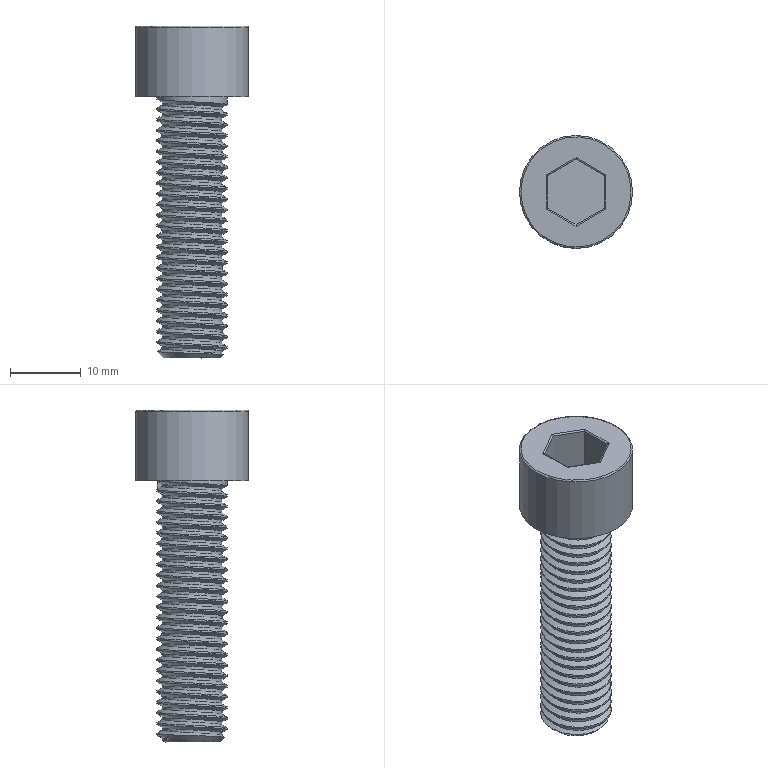Part | STEP file | Tube feed_id1626_x_t | 1 solid | 25 faces | box 16 x 16 x 47 mm | volume 3975 mm3 | plane 11 | cylinder 9 | spline 3 | cone 1 | torus 1 | commonest cylinder face diameters 0.4 x6 8.5 x1 10 x1 16 x1